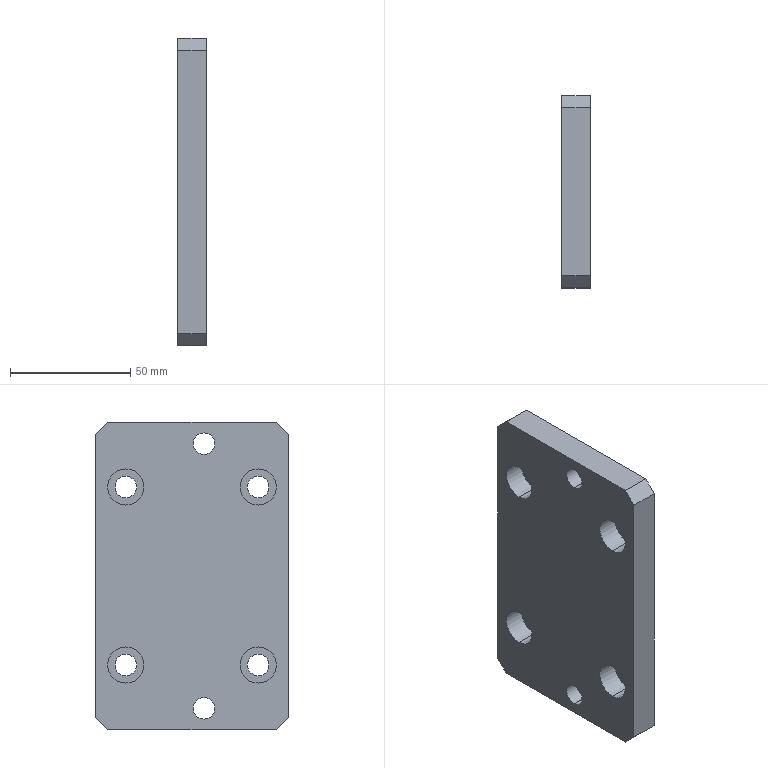Part | SolidWorks | features HoleWzd 2, Chamfer 1, Extrusion 1 | 1 solid | 34 faces | box 12 x 80 x 128 mm | volume 113628 mm3 | cylinder 20 | plane 14 | commonest cylinder face diameters 9 x12 15 x8
STEP:
#1=CARTESIAN_POINT('',(0.,-5.,59.5));
#2=VERTEX_POINT('',#1);
#3=CARTESIAN_POINT('',(0.,-5.,50.5));
#4=VERTEX_POINT('',#3);
#5=CARTESIAN_POINT('',(0.,-5.,55.));
#6=DIRECTION('',(1.,0.,0.));
#7=DIRECTION('',(0.,0.,-1.));
#8=AXIS2_PLACEMENT_3D('',#5,#6,#7);
#9=CIRCLE('',#8,4.5);
#10=EDGE_CURVE('',#2,#4,#9,.T.);
#11=ORIENTED_EDGE('',*,*,#10,.F.);
#12=CARTESIAN_POINT('',(12.,-5.,59.5));
#13=VERTEX_POINT('',#12);
#14=CARTESIAN_POINT('',(12.,-5.,59.5));
#15=DIRECTION('',(1.,0.,0.));
#16=VECTOR('',#15,1000.);
#17=LINE('',#14,#16);
#18=EDGE_CURVE('',#2,#13,#17,.T.);
#19=ORIENTED_EDGE('',*,*,#18,.T.);
#20=CARTESIAN_POINT('',(12.,-5.,50.5));
#21=VERTEX_POINT('',#20);
#22=CARTESIAN_POINT('',(12.,-5.,55.));
#23=DIRECTION('',(1.,0.,0.));
#24=DIRECTION('',(0.,0.,-1.));
#25=AXIS2_PLACEMENT_3D('',#22,#23,#24);
#26=CIRCLE('',#25,4.5);
#27=EDGE_CURVE('',#13,#21,#26,.T.);
#28=ORIENTED_EDGE('',*,*,#27,.T.);
#29=CARTESIAN_POINT('',(12.,-5.,50.5));
#30=DIRECTION('',(1.,0.,0.));
#31=VECTOR('',#30,1000.);
#32=LINE('',#29,#31);
#33=EDGE_CURVE('',#4,#21,#32,.T.);
#34=ORIENTED_EDGE('',*,*,#33,.F.);
#35=EDGE_LOOP('',(#11,#19,#28,#34));
#36=FACE_OUTER_BOUND('',#35,.T.);
#37=CARTESIAN_POINT('',(12.,-5.,55.));
#38=DIRECTION('',(1.,0.,0.));
#39=DIRECTION('',(0.,0.,-1.));
#40=AXIS2_PLACEMENT_3D('',#37,#38,#39);
#41=CYLINDRICAL_SURFACE('',#40,4.5);
#42=ADVANCED_FACE('',(#36),#41,.F.);
#43=CARTESIAN_POINT('',(0.,-5.,-50.5));
#44=VERTEX_POINT('',#43);
#45=CARTESIAN_POINT('',(0.,-5.,-59.5));
#46=VERTEX_POINT('',#45);
#47=CARTESIAN_POINT('',(0.,-5.,-55.));
#48=DIRECTION('',(1.,0.,0.));
#49=DIRECTION('',(0.,0.,-1.));
#50=AXIS2_PLACEMENT_3D('',#47,#48,#49);
#51=CIRCLE('',#50,4.5);
#52=EDGE_CURVE('',#44,#46,#51,.T.);
#53=ORIENTED_EDGE('',*,*,#52,.F.);
#54=CARTESIAN_POINT('',(12.,-5.,-50.5));
#55=VERTEX_POINT('',#54);
#56=CARTESIAN_POINT('',(12.,-5.,-50.5));
#57=DIRECTION('',(1.,0.,0.));
#58=VECTOR('',#57,1000.);
#59=LINE('',#56,#58);
#60=EDGE_CURVE('',#44,#55,#59,.T.);
#61=ORIENTED_EDGE('',*,*,#60,.T.);
#62=CARTESIAN_POINT('',(12.,-5.,-59.5));
#63=VERTEX_POINT('',#62);
#64=CARTESIAN_POINT('',(12.,-5.,-55.));
#65=DIRECTION('',(1.,0.,0.));
#66=DIRECTION('',(0.,0.,-1.));
#67=AXIS2_PLACEMENT_3D('',#64,#65,#66);
#68=CIRCLE('',#67,4.5);
#69=EDGE_CURVE('',#55,#63,#68,.T.);
#70=ORIENTED_EDGE('',*,*,#69,.T.);
#71=CARTESIAN_POINT('',(12.,-5.,-59.5));
#72=DIRECTION('',(1.,0.,0.));
#73=VECTOR('',#72,1000.);
#74=LINE('',#71,#73);
#75=EDGE_CURVE('',#46,#63,#74,.T.);
#76=ORIENTED_EDGE('',*,*,#75,.F.);
#77=EDGE_LOOP('',(#53,#61,#70,#76));
#78=FACE_OUTER_BOUND('',#77,.T.);
#79=CARTESIAN_POINT('',(12.,-5.,-55.));
#80=DIRECTION('',(1.,0.,0.));
#81=DIRECTION('',(0.,0.,-1.));
#82=AXIS2_PLACEMENT_3D('',#79,#80,#81);
#83=CYLINDRICAL_SURFACE('',#82,4.5);
#84=ADVANCED_FACE('',(#78),#83,.F.);
#85=CARTESIAN_POINT('',(9.,27.5,-44.5));
#86=VERTEX_POINT('',#85);
#87=CARTESIAN_POINT('',(9.,27.5,-29.5));
#88=VERTEX_POINT('',#87);
#89=CARTESIAN_POINT('',(9.,27.5,-37.));
#90=DIRECTION('',(-1.,0.,0.));
#91=DIRECTION('',(0.,0.,1.));
#92=AXIS2_PLACEMENT_3D('',#89,#90,#91);
#93=CIRCLE('',#92,7.5);
#94=EDGE_CURVE('',#86,#88,#93,.T.);
#95=ORIENTED_EDGE('',*,*,#94,.F.);
#96=CARTESIAN_POINT('',(0.,27.5,-44.5));
#97=VERTEX_POINT('',#96);
#98=CARTESIAN_POINT('',(0.,27.5,-44.5));
#99=DIRECTION('',(-1.,0.,0.));
#100=VECTOR('',#99,1000.);
#101=LINE('',#98,#100);
#102=EDGE_CURVE('',#86,#97,#101,.T.);
#103=ORIENTED_EDGE('',*,*,#102,.T.);
#104=CARTESIAN_POINT('',(0.,27.5,-29.5));
#105=VERTEX_POINT('',#104);
#106=CARTESIAN_POINT('',(0.,27.5,-37.));
#107=DIRECTION('',(-1.,0.,0.));
#108=DIRECTION('',(0.,0.,1.));
#109=AXIS2_PLACEMENT_3D('',#106,#107,#108);
#110=CIRCLE('',#109,7.5);
#111=EDGE_CURVE('',#97,#105,#110,.T.);
#112=ORIENTED_EDGE('',*,*,#111,.T.);
#113=CARTESIAN_POINT('',(0.,27.5,-29.5));
#114=DIRECTION('',(-1.,0.,0.));
#115=VECTOR('',#114,1000.);
#116=LINE('',#113,#115);
#117=EDGE_CURVE('',#88,#105,#116,.T.);
#118=ORIENTED_EDGE('',*,*,#117,.F.);
#119=EDGE_LOOP('',(#95,#103,#112,#118));
#120=FACE_OUTER_BOUND('',#119,.T.);
#121=CARTESIAN_POINT('',(0.,27.5,-37.));
#122=DIRECTION('',(-1.,0.,0.));
#123=DIRECTION('',(0.,0.,1.));
#124=AXIS2_PLACEMENT_3D('',#121,#122,#123);
#125=CYLINDRICAL_SURFACE('',#124,7.5);
#126=ADVANCED_FACE('',(#120),#125,.F.);
#127=CARTESIAN_POINT('',(12.,27.5,-41.5));
#128=VERTEX_POINT('',#127);
#129=CARTESIAN_POINT('',(12.,27.5,-32.5));
#130=VERTEX_POINT('',#129);
#131=CARTESIAN_POINT('',(12.,27.5,-37.));
#132=DIRECTION('',(-1.,0.,0.));
#133=DIRECTION('',(0.,0.,1.));
#134=AXIS2_PLACEMENT_3D('',#131,#132,#133);
#135=CIRCLE('',#134,4.5);
#136=EDGE_CURVE('',#128,#130,#135,.T.);
#137=ORIENTED_EDGE('',*,*,#136,.F.);
#138=CARTESIAN_POINT('',(9.,27.5,-41.5));
#139=VERTEX_POINT('',#138);
#140=CARTESIAN_POINT('',(0.,27.5,-41.5));
#141=DIRECTION('',(-1.,0.,0.));
#142=VECTOR('',#141,1000.);
#143=LINE('',#140,#142);
#144=EDGE_CURVE('',#128,#139,#143,.T.);
#145=ORIENTED_EDGE('',*,*,#144,.T.);
#146=CARTESIAN_POINT('',(9.,27.5,-32.5));
#147=VERTEX_POINT('',#146);
#148=CARTESIAN_POINT('',(9.,27.5,-37.));
#149=DIRECTION('',(-1.,0.,0.));
#150=DIRECTION('',(0.,0.,1.));
#151=AXIS2_PLACEMENT_3D('',#148,#149,#150);
#152=CIRCLE('',#151,4.5);
#153=EDGE_CURVE('',#139,#147,#152,.T.);
#154=ORIENTED_EDGE('',*,*,#153,.T.);
#155=CARTESIAN_POINT('',(0.,27.5,-32.5));
#156=DIRECTION('',(-1.,0.,0.));
#157=VECTOR('',#156,1000.);
#158=LINE('',#155,#157);
#159=EDGE_CURVE('',#130,#147,#158,.T.);
#160=ORIENTED_EDGE('',*,*,#159,.F.);
#161=EDGE_LOOP('',(#137,#145,#154,#160));
#162=FACE_OUTER_BOUND('',#161,.T.);
#163=CARTESIAN_POINT('',(0.,27.5,-37.));
#164=DIRECTION('',(-1.,0.,0.));
#165=DIRECTION('',(0.,0.,1.));
#166=AXIS2_PLACEMENT_3D('',#163,#164,#165);
#167=CYLINDRICAL_SURFACE('',#166,4.5);
#168=ADVANCED_FACE('',(#162),#167,.F.);
#169=CARTESIAN_POINT('',(9.,-27.5,-44.5));
#170=VERTEX_POINT('',#169);
#171=CARTESIAN_POINT('',(9.,-27.5,-29.5));
#172=VERTEX_POINT('',#171);
#173=CARTESIAN_POINT('',(9.,-27.5,-37.));
#174=DIRECTION('',(-1.,0.,0.));
#175=DIRECTION('',(0.,0.,1.));
#176=AXIS2_PLACEMENT_3D('',#173,#174,#175);
#177=CIRCLE('',#176,7.5);
#178=EDGE_CURVE('',#170,#172,#177,.T.);
#179=ORIENTED_EDGE('',*,*,#178,.F.);
#180=CARTESIAN_POINT('',(0.,-27.5,-44.5));
#181=VERTEX_POINT('',#180);
#182=CARTESIAN_POINT('',(0.,-27.5,-44.5));
#183=DIRECTION('',(-1.,0.,0.));
#184=VECTOR('',#183,1000.);
#185=LINE('',#182,#184);
#186=EDGE_CURVE('',#170,#181,#185,.T.);
#187=ORIENTED_EDGE('',*,*,#186,.T.);
#188=CARTESIAN_POINT('',(0.,-27.5,-29.5));
#189=VERTEX_POINT('',#188);
#190=CARTESIAN_POINT('',(0.,-27.5,-37.));
#191=DIRECTION('',(-1.,0.,0.));
#192=DIRECTION('',(0.,0.,1.));
#193=AXIS2_PLACEMENT_3D('',#190,#191,#192);
#194=CIRCLE('',#193,7.5);
#195=EDGE_CURVE('',#181,#189,#194,.T.);
#196=ORIENTED_EDGE('',*,*,#195,.T.);
#197=CARTESIAN_POINT('',(0.,-27.5,-29.5));
#198=DIRECTION('',(-1.,0.,0.));
#199=VECTOR('',#198,1000.);
#200=LINE('',#197,#199);
#201=EDGE_CURVE('',#172,#189,#200,.T.);
#202=ORIENTED_EDGE('',*,*,#201,.F.);
#203=EDGE_LOOP('',(#179,#187,#196,#202));
#204=FACE_OUTER_BOUND('',#203,.T.);
#205=CARTESIAN_POINT('',(0.,-27.5,-37.));
#206=DIRECTION('',(-1.,0.,0.));
#207=DIRECTION('',(0.,0.,1.));
#208=AXIS2_PLACEMENT_3D('',#205,#206,#207);
#209=CYLINDRICAL_SURFACE('',#208,7.5);
#210=ADVANCED_FACE('',(#204),#209,.F.);
#211=CARTESIAN_POINT('',(12.,-27.5,-41.5));
#212=VERTEX_POINT('',#211);
#213=CARTESIAN_POINT('',(12.,-27.5,-32.5));
#214=VERTEX_POINT('',#213);
#215=CARTESIAN_POINT('',(12.,-27.5,-37.));
#216=DIRECTION('',(-1.,0.,0.));
#217=DIRECTION('',(0.,0.,1.));
#218=AXIS2_PLACEMENT_3D('',#215,#216,#217);
#219=CIRCLE('',#218,4.5);
#220=EDGE_CURVE('',#212,#214,#219,.T.);
#221=ORIENTED_EDGE('',*,*,#220,.F.);
#222=CARTESIAN_POINT('',(9.,-27.5,-41.5));
#223=VERTEX_POINT('',#222);
#224=CARTESIAN_POINT('',(0.,-27.5,-41.5));
#225=DIRECTION('',(-1.,0.,0.));
#226=VECTOR('',#225,1000.);
#227=LINE('',#224,#226);
#228=EDGE_CURVE('',#212,#223,#227,.T.);
#229=ORIENTED_EDGE('',*,*,#228,.T.);
#230=CARTESIAN_POINT('',(9.,-27.5,-32.5));
#231=VERTEX_POINT('',#230);
#232=CARTESIAN_POINT('',(9.,-27.5,-37.));
#233=DIRECTION('',(-1.,0.,0.));
#234=DIRECTION('',(0.,0.,1.));
#235=AXIS2_PLACEMENT_3D('',#232,#233,#234);
#236=CIRCLE('',#235,4.5);
#237=EDGE_CURVE('',#223,#231,#236,.T.);
#238=ORIENTED_EDGE('',*,*,#237,.T.);
#239=CARTESIAN_POINT('',(0.,-27.5,-32.5));
#240=DIRECTION('',(-1.,0.,0.));
#241=VECTOR('',#240,1000.);
#242=LINE('',#239,#241);
#243=EDGE_CURVE('',#214,#231,#242,.T.);
#244=ORIENTED_EDGE('',*,*,#243,.F.);
#245=EDGE_LOOP('',(#221,#229,#238,#244));
#246=FACE_OUTER_BOUND('',#245,.T.);
#247=CARTESIAN_POINT('',(0.,-27.5,-37.));
#248=DIRECTION('',(-1.,0.,0.));
#249=DIRECTION('',(0.,0.,1.));
#250=AXIS2_PLACEMENT_3D('',#247,#248,#249);
#251=CYLINDRICAL_SURFACE('',#250,4.5);
#252=ADVANCED_FACE('',(#246),#251,.F.);
#253=CARTESIAN_POINT('',(9.,27.5,29.5));
#254=VERTEX_POINT('',#253);
#255=CARTESIAN_POINT('',(9.,27.5,44.5));
#256=VERTEX_POINT('',#255);
#257=CARTESIAN_POINT('',(9.,27.5,37.));
#258=DIRECTION('',(-1.,0.,0.));
#259=DIRECTION('',(0.,0.,1.));
#260=AXIS2_PLACEMENT_3D('',#257,#258,#259);
#261=CIRCLE('',#260,7.5);
#262=EDGE_CURVE('',#254,#256,#261,.T.);
#263=ORIENTED_EDGE('',*,*,#262,.F.);
#264=CARTESIAN_POINT('',(0.,27.5,29.5));
#265=VERTEX_POINT('',#264);
#266=CARTESIAN_POINT('',(0.,27.5,29.5));
#267=DIRECTION('',(-1.,0.,0.));
#268=VECTOR('',#267,1000.);
#269=LINE('',#266,#268);
#270=EDGE_CURVE('',#254,#265,#269,.T.);
#271=ORIENTED_EDGE('',*,*,#270,.T.);
#272=CARTESIAN_POINT('',(0.,27.5,44.5));
#273=VERTEX_POINT('',#272);
#274=CARTESIAN_POINT('',(0.,27.5,37.));
#275=DIRECTION('',(-1.,0.,0.));
#276=DIRECTION('',(0.,0.,1.));
#277=AXIS2_PLACEMENT_3D('',#274,#275,#276);
#278=CIRCLE('',#277,7.5);
#279=EDGE_CURVE('',#265,#273,#278,.T.);
#280=ORIENTED_EDGE('',*,*,#279,.T.);
#281=CARTESIAN_POINT('',(0.,27.5,44.5));
#282=DIRECTION('',(-1.,0.,0.));
#283=VECTOR('',#282,1000.);
#284=LINE('',#281,#283);
#285=EDGE_CURVE('',#256,#273,#284,.T.);
#286=ORIENTED_EDGE('',*,*,#285,.F.);
#287=EDGE_LOOP('',(#263,#271,#280,#286));
#288=FACE_OUTER_BOUND('',#287,.T.);
#289=CARTESIAN_POINT('',(0.,27.5,37.));
#290=DIRECTION('',(-1.,0.,0.));
#291=DIRECTION('',(0.,0.,1.));
#292=AXIS2_PLACEMENT_3D('',#289,#290,#291);
#293=CYLINDRICAL_SURFACE('',#292,7.5);
#294=ADVANCED_FACE('',(#288),#293,.F.);
#295=CARTESIAN_POINT('',(12.,27.5,32.5));
#296=VERTEX_POINT('',#295);
#297=CARTESIAN_POINT('',(12.,27.5,41.5));
#298=VERTEX_POINT('',#297);
#299=CARTESIAN_POINT('',(12.,27.5,37.));
#300=DIRECTION('',(-1.,0.,0.));
#301=DIRECTION('',(0.,0.,1.));
#302=AXIS2_PLACEMENT_3D('',#299,#300,#301);
#303=CIRCLE('',#302,4.5);
#304=EDGE_CURVE('',#296,#298,#303,.T.);
#305=ORIENTED_EDGE('',*,*,#304,.F.);
#306=CARTESIAN_POINT('',(9.,27.5,32.5));
#307=VERTEX_POINT('',#306);
#308=CARTESIAN_POINT('',(0.,27.5,32.5));
#309=DIRECTION('',(-1.,0.,0.));
#310=VECTOR('',#309,1000.);
#311=LINE('',#308,#310);
#312=EDGE_CURVE('',#296,#307,#311,.T.);
#313=ORIENTED_EDGE('',*,*,#312,.T.);
#314=CARTESIAN_POINT('',(9.,27.5,41.5));
#315=VERTEX_POINT('',#314);
#316=CARTESIAN_POINT('',(9.,27.5,37.));
#317=DIRECTION('',(-1.,0.,0.));
#318=DIRECTION('',(0.,0.,1.));
#319=AXIS2_PLACEMENT_3D('',#316,#317,#318);
#320=CIRCLE('',#319,4.5);
#321=EDGE_CURVE('',#307,#315,#320,.T.);
#322=ORIENTED_EDGE('',*,*,#321,.T.);
#323=CARTESIAN_POINT('',(0.,27.5,41.5));
#324=DIRECTION('',(-1.,0.,0.));
#325=VECTOR('',#324,1000.);
#326=LINE('',#323,#325);
#327=EDGE_CURVE('',#298,#315,#326,.T.);
#328=ORIENTED_EDGE('',*,*,#327,.F.);
#329=EDGE_LOOP('',(#305,#313,#322,#328));
#330=FACE_OUTER_BOUND('',#329,.T.);
#331=CARTESIAN_POINT('',(0.,27.5,37.));
#332=DIRECTION('',(-1.,0.,0.));
#333=DIRECTION('',(0.,0.,1.));
#334=AXIS2_PLACEMENT_3D('',#331,#332,#333);
#335=CYLINDRICAL_SURFACE('',#334,4.5);
#336=ADVANCED_FACE('',(#330),#335,.F.);
#337=CARTESIAN_POINT('',(9.,-27.5,29.5));
#338=VERTEX_POINT('',#337);
#339=CARTESIAN_POINT('',(9.,-27.5,44.5));
#340=VERTEX_POINT('',#339);
#341=CARTESIAN_POINT('',(9.,-27.5,37.));
#342=DIRECTION('',(-1.,0.,0.));
#343=DIRECTION('',(0.,0.,1.));
#344=AXIS2_PLACEMENT_3D('',#341,#342,#343);
#345=CIRCLE('',#344,7.5);
#346=EDGE_CURVE('',#338,#340,#345,.T.);
#347=ORIENTED_EDGE('',*,*,#346,.F.);
#348=CARTESIAN_POINT('',(0.,-27.5,29.5));
#349=VERTEX_POINT('',#348);
#350=CARTESIAN_POINT('',(0.,-27.5,29.5));
#351=DIRECTION('',(-1.,0.,0.));
#352=VECTOR('',#351,1000.);
#353=LINE('',#350,#352);
#354=EDGE_CURVE('',#338,#349,#353,.T.);
#355=ORIENTED_EDGE('',*,*,#354,.T.);
#356=CARTESIAN_POINT('',(0.,-27.5,44.5));
#357=VERTEX_POINT('',#356);
#358=CARTESIAN_POINT('',(0.,-27.5,37.));
#359=DIRECTION('',(-1.,0.,0.));
#360=DIRECTION('',(0.,0.,1.));
#361=AXIS2_PLACEMENT_3D('',#358,#359,#360);
#362=CIRCLE('',#361,7.5);
#363=EDGE_CURVE('',#349,#357,#362,.T.);
#364=ORIENTED_EDGE('',*,*,#363,.T.);
#365=CARTESIAN_POINT('',(0.,-27.5,44.5));
#366=DIRECTION('',(-1.,0.,0.));
#367=VECTOR('',#366,1000.);
#368=LINE('',#365,#367);
#369=EDGE_CURVE('',#340,#357,#368,.T.);
#370=ORIENTED_EDGE('',*,*,#369,.F.);
#371=EDGE_LOOP('',(#347,#355,#364,#370));
#372=FACE_OUTER_BOUND('',#371,.T.);
#373=CARTESIAN_POINT('',(0.,-27.5,37.));
#374=DIRECTION('',(-1.,0.,0.));
#375=DIRECTION('',(0.,0.,1.));
#376=AXIS2_PLACEMENT_3D('',#373,#374,#375);
#377=CYLINDRICAL_SURFACE('',#376,7.5);
#378=ADVANCED_FACE('',(#372),#377,.F.);
#379=CARTESIAN_POINT('',(12.,-27.5,32.5));
#380=VERTEX_POINT('',#379);
#381=CARTESIAN_POINT('',(12.,-27.5,41.5));
#382=VERTEX_POINT('',#381);
#383=CARTESIAN_POINT('',(12.,-27.5,37.));
#384=DIRECTION('',(-1.,0.,0.));
#385=DIRECTION('',(0.,0.,1.));
#386=AXIS2_PLACEMENT_3D('',#383,#384,#385);
#387=CIRCLE('',#386,4.5);
#388=EDGE_CURVE('',#380,#382,#387,.T.);
#389=ORIENTED_EDGE('',*,*,#388,.F.);
#390=CARTESIAN_POINT('',(9.,-27.5,32.5));
#391=VERTEX_POINT('',#390);
#392=CARTESIAN_POINT('',(0.,-27.5,32.5));
#393=DIRECTION('',(-1.,0.,0.));
#394=VECTOR('',#393,1000.);
#395=LINE('',#392,#394);
#396=EDGE_CURVE('',#380,#391,#395,.T.);
#397=ORIENTED_EDGE('',*,*,#396,.T.);
#398=CARTESIAN_POINT('',(9.,-27.5,41.5));
#399=VERTEX_POINT('',#398);
#400=CARTESIAN_POINT('',(9.,-27.5,37.));
#401=DIRECTION('',(-1.,0.,0.));
#402=DIRECTION('',(0.,0.,1.));
#403=AXIS2_PLACEMENT_3D('',#400,#401,#402);
#404=CIRCLE('',#403,4.5);
#405=EDGE_CURVE('',#391,#399,#404,.T.);
#406=ORIENTED_EDGE('',*,*,#405,.T.);
#407=CARTESIAN_POINT('',(0.,-27.5,41.5));
#408=DIRECTION('',(-1.,0.,0.));
#409=VECTOR('',#408,1000.);
#410=LINE('',#407,#409);
#411=EDGE_CURVE('',#382,#399,#410,.T.);
#412=ORIENTED_EDGE('',*,*,#411,.F.);
#413=EDGE_LOOP('',(#389,#397,#406,#412));
#414=FACE_OUTER_BOUND('',#413,.T.);
#415=CARTESIAN_POINT('',(0.,-27.5,37.));
#416=DIRECTION('',(-1.,0.,0.));
#417=DIRECTION('',(0.,0.,1.));
#418=AXIS2_PLACEMENT_3D('',#415,#416,#417);
#419=CYLINDRICAL_SURFACE('',#418,4.5);
#420=ADVANCED_FACE('',(#414),#419,.F.);
#421=CARTESIAN_POINT('',(12.,-35.,-64.));
#422=VERTEX_POINT('',#421);
#423=CARTESIAN_POINT('',(12.,35.,-64.));
#424=VERTEX_POINT('',#423);
#425=CARTESIAN_POINT('',(12.,40.,-64.));
#426=DIRECTION('',(0.,1.,0.));
#427=VECTOR('',#426,1000.);
#428=LINE('',#425,#427);
#429=EDGE_CURVE('',#422,#424,#428,.T.);
#430=ORIENTED_EDGE('',*,*,#429,.F.);
#431=CARTESIAN_POINT('',(0.,-35.,-64.));
#432=VERTEX_POINT('',#431);
#433=CARTESIAN_POINT('',(12.,-35.,-64.));
#434=DIRECTION('',(-1.,0.,0.));
#435=VECTOR('',#434,1000.);
#436=LINE('',#433,#435);
#437=EDGE_CURVE('',#422,#432,#436,.T.);
#438=ORIENTED_EDGE('',*,*,#437,.T.);
#439=CARTESIAN_POINT('',(0.,35.,-64.));
#440=VERTEX_POINT('',#439);
#441=CARTESIAN_POINT('',(0.,40.,-64.));
#442=DIRECTION('',(0.,1.,0.));
#443=VECTOR('',#442,1000.);
#444=LINE('',#441,#443);
#445=EDGE_CURVE('',#432,#440,#444,.T.);
#446=ORIENTED_EDGE('',*,*,#445,.T.);
#447=CARTESIAN_POINT('',(12.,35.,-64.));
#448=DIRECTION('',(1.,0.,0.));
#449=VECTOR('',#448,1000.);
#450=LINE('',#447,#449);
#451=EDGE_CURVE('',#440,#424,#450,.T.);
#452=ORIENTED_EDGE('',*,*,#451,.T.);
#453=EDGE_LOOP('',(#430,#438,#446,#452));
#454=FACE_OUTER_BOUND('',#453,.T.);
#455=CARTESIAN_POINT('',(12.,40.,-64.));
#456=DIRECTION('',(0.,0.,1.));
#457=DIRECTION('',(1.,0.,0.));
#458=AXIS2_PLACEMENT_3D('',#455,#456,#457);
#459=PLANE('',#458);
#460=ADVANCED_FACE('',(#454),#459,.F.);
#461=CARTESIAN_POINT('',(12.,40.,-59.));
#462=VERTEX_POINT('',#461);
#463=CARTESIAN_POINT('',(12.,40.,59.));
#464=VERTEX_POINT('',#463);
#465=CARTESIAN_POINT('',(12.,40.,64.));
#466=DIRECTION('',(0.,0.,1.));
#467=VECTOR('',#466,1000.);
#468=LINE('',#465,#467);
#469=EDGE_CURVE('',#462,#464,#468,.T.);
#470=ORIENTED_EDGE('',*,*,#469,.F.);
#471=CARTESIAN_POINT('',(0.,40.,-59.));
#472=VERTEX_POINT('',#471);
#473=CARTESIAN_POINT('',(12.,40.,-59.));
#474=DIRECTION('',(-1.,0.,0.));
#475=VECTOR('',#474,1000.);
#476=LINE('',#473,#475);
#477=EDGE_CURVE('',#462,#472,#476,.T.);
#478=ORIENTED_EDGE('',*,*,#477,.T.);
#479=CARTESIAN_POINT('',(0.,40.,59.));
#480=VERTEX_POINT('',#479);
#481=CARTESIAN_POINT('',(0.,40.,64.));
#482=DIRECTION('',(0.,0.,1.));
#483=VECTOR('',#482,1000.);
#484=LINE('',#481,#483);
#485=EDGE_CURVE('',#472,#480,#484,.T.);
#486=ORIENTED_EDGE('',*,*,#485,.T.);
#487=CARTESIAN_POINT('',(12.,40.,59.));
#488=DIRECTION('',(1.,0.,0.));
#489=VECTOR('',#488,1000.);
#490=LINE('',#487,#489);
#491=EDGE_CURVE('',#480,#464,#490,.T.);
#492=ORIENTED_EDGE('',*,*,#491,.T.);
#493=EDGE_LOOP('',(#470,#478,#486,#492));
#494=FACE_OUTER_BOUND('',#493,.T.);
#495=CARTESIAN_POINT('',(12.,40.,64.));
#496=DIRECTION('',(0.,-1.,0.));
#497=DIRECTION('',(0.,0.,-1.));
#498=AXIS2_PLACEMENT_3D('',#495,#496,#497);
#499=PLANE('',#498);
#500=ADVANCED_FACE('',(#494),#499,.F.);
#501=CARTESIAN_POINT('',(0.,35.,64.));
#502=VERTEX_POINT('',#501);
#503=CARTESIAN_POINT('',(0.,-35.,64.));
#504=VERTEX_POINT('',#503);
#505=CARTESIAN_POINT('',(0.,40.,64.));
#506=DIRECTION('',(0.,-1.,0.));
#507=VECTOR('',#506,1000.);
#508=LINE('',#505,#507);
#509=EDGE_CURVE('',#502,#504,#508,.T.);
#510=ORIENTED_EDGE('',*,*,#509,.T.);
#511=CARTESIAN_POINT('',(12.,-35.,64.));
#512=VERTEX_POINT('',#511);
#513=CARTESIAN_POINT('',(12.,-35.,64.));
#514=DIRECTION('',(1.,0.,0.));
#515=VECTOR('',#514,1000.);
#516=LINE('',#513,#515);
#517=EDGE_CURVE('',#504,#512,#516,.T.);
#518=ORIENTED_EDGE('',*,*,#517,.T.);
#519=CARTESIAN_POINT('',(12.,35.,64.));
#520=VERTEX_POINT('',#519);
#521=CARTESIAN_POINT('',(12.,40.,64.));
#522=DIRECTION('',(0.,-1.,0.));
#523=VECTOR('',#522,1000.);
#524=LINE('',#521,#523);
#525=EDGE_CURVE('',#520,#512,#524,.T.);
#526=ORIENTED_EDGE('',*,*,#525,.F.);
#527=CARTESIAN_POINT('',(12.,35.,64.));
#528=DIRECTION('',(-1.,0.,0.));
#529=VECTOR('',#528,1000.);
#530=LINE('',#527,#529);
#531=EDGE_CURVE('',#520,#502,#530,.T.);
#532=ORIENTED_EDGE('',*,*,#531,.T.);
#533=EDGE_LOOP('',(#510,#518,#526,#532));
#534=FACE_OUTER_BOUND('',#533,.T.);
#535=CARTESIAN_POINT('',(12.,40.,64.));
#536=DIRECTION('',(0.,0.,-1.));
#537=DIRECTION('',(0.,1.,0.));
#538=AXIS2_PLACEMENT_3D('',#535,#536,#537);
#539=PLANE('',#538);
#540=ADVANCED_FACE('',(#534),#539,.F.);
#541=CARTESIAN_POINT('',(12.,-40.,59.));
#542=VERTEX_POINT('',#541);
#543=CARTESIAN_POINT('',(12.,-40.,-59.));
#544=VERTEX_POINT('',#543);
#545=CARTESIAN_POINT('',(12.,-40.,64.));
#546=DIRECTION('',(0.,0.,-1.));
#547=VECTOR('',#546,1000.);
#548=LINE('',#545,#547);
#549=EDGE_CURVE('',#542,#544,#548,.T.);
#550=ORIENTED_EDGE('',*,*,#549,.F.);
#551=CARTESIAN_POINT('',(0.,-40.,59.));
#552=VERTEX_POINT('',#551);
#553=CARTESIAN_POINT('',(12.,-40.,59.));
#554=DIRECTION('',(-1.,0.,0.));
#555=VECTOR('',#554,1000.);
#556=LINE('',#553,#555);
#557=EDGE_CURVE('',#542,#552,#556,.T.);
#558=ORIENTED_EDGE('',*,*,#557,.T.);
#559=CARTESIAN_POINT('',(0.,-40.,-59.));
#560=VERTEX_POINT('',#559);
#561=CARTESIAN_POINT('',(0.,-40.,64.));
#562=DIRECTION('',(0.,0.,-1.));
#563=VECTOR('',#562,1000.);
#564=LINE('',#561,#563);
#565=EDGE_CURVE('',#552,#560,#564,.T.);
#566=ORIENTED_EDGE('',*,*,#565,.T.);
#567=CARTESIAN_POINT('',(12.,-40.,-59.));
#568=DIRECTION('',(1.,0.,0.));
#569=VECTOR('',#568,1000.);
#570=LINE('',#567,#569);
#571=EDGE_CURVE('',#560,#544,#570,.T.);
#572=ORIENTED_EDGE('',*,*,#571,.T.);
#573=EDGE_LOOP('',(#550,#558,#566,#572));
#574=FACE_OUTER_BOUND('',#573,.T.);
#575=CARTESIAN_POINT('',(12.,-40.,64.));
#576=DIRECTION('',(0.,1.,0.));
#577=DIRECTION('',(0.,0.,1.));
#578=AXIS2_PLACEMENT_3D('',#575,#576,#577);
#579=PLANE('',#578);
#580=ADVANCED_FACE('',(#574),#579,.F.);
#581=CARTESIAN_POINT('',(12.,-5.,55.));
#582=DIRECTION('',(1.,0.,0.));
#583=DIRECTION('',(0.,0.,-1.));
#584=AXIS2_PLACEMENT_3D('',#581,#582,#583);
#585=CIRCLE('',#584,4.5);
#586=EDGE_CURVE('',#21,#13,#585,.T.);
#587=ORIENTED_EDGE('',*,*,#586,.F.);
#588=ORIENTED_EDGE('',*,*,#27,.F.);
#589=EDGE_LOOP('',(#587,#588));
#590=FACE_BOUND('',#589,.T.);
#591=CARTESIAN_POINT('',(12.,-5.,-55.));
#592=DIRECTION('',(1.,0.,0.));
#593=DIRECTION('',(0.,0.,-1.));
#594=AXIS2_PLACEMENT_3D('',#591,#592,#593);
#595=CIRCLE('',#594,4.5);
#596=EDGE_CURVE('',#63,#55,#595,.T.);
#597=ORIENTED_EDGE('',*,*,#596,.F.);
#598=ORIENTED_EDGE('',*,*,#69,.F.);
#599=EDGE_LOOP('',(#597,#598));
#600=FACE_BOUND('',#599,.T.);
#601=CARTESIAN_POINT('',(12.,27.5,-37.));
#602=DIRECTION('',(-1.,0.,0.));
#603=DIRECTION('',(0.,0.,1.));
#604=AXIS2_PLACEMENT_3D('',#601,#602,#603);
#605=CIRCLE('',#604,4.5);
#606=EDGE_CURVE('',#130,#128,#605,.T.);
#607=ORIENTED_EDGE('',*,*,#606,.T.);
#608=ORIENTED_EDGE('',*,*,#136,.T.);
#609=EDGE_LOOP('',(#607,#608));
#610=FACE_BOUND('',#609,.T.);
#611=CARTESIAN_POINT('',(12.,-27.5,-37.));
#612=DIRECTION('',(-1.,0.,0.));
#613=DIRECTION('',(0.,0.,1.));
#614=AXIS2_PLACEMENT_3D('',#611,#612,#613);
#615=CIRCLE('',#614,4.5);
#616=EDGE_CURVE('',#214,#212,#615,.T.);
#617=ORIENTED_EDGE('',*,*,#616,.T.);
#618=ORIENTED_EDGE('',*,*,#220,.T.);
#619=EDGE_LOOP('',(#617,#618));
#620=FACE_BOUND('',#619,.T.);
#621=CARTESIAN_POINT('',(12.,27.5,37.));
#622=DIRECTION('',(-1.,0.,0.));
#623=DIRECTION('',(0.,0.,1.));
#624=AXIS2_PLACEMENT_3D('',#621,#622,#623);
#625=CIRCLE('',#624,4.5);
#626=EDGE_CURVE('',#298,#296,#625,.T.);
#627=ORIENTED_EDGE('',*,*,#626,.T.);
#628=ORIENTED_EDGE('',*,*,#304,.T.);
#629=EDGE_LOOP('',(#627,#628));
#630=FACE_BOUND('',#629,.T.);
#631=CARTESIAN_POINT('',(12.,-27.5,37.));
#632=DIRECTION('',(-1.,0.,0.));
#633=DIRECTION('',(0.,0.,1.));
#634=AXIS2_PLACEMENT_3D('',#631,#632,#633);
#635=CIRCLE('',#634,4.5);
#636=EDGE_CURVE('',#382,#380,#635,.T.);
#637=ORIENTED_EDGE('',*,*,#636,.T.);
#638=ORIENTED_EDGE('',*,*,#388,.T.);
#639=EDGE_LOOP('',(#637,#638));
#640=FACE_BOUND('',#639,.T.);
#641=ORIENTED_EDGE('',*,*,#525,.T.);
#642=CARTESIAN_POINT('',(12.,-49.5,49.5));
#643=DIRECTION('',(0.,-0.7071,-0.7071));
#644=VECTOR('',#643,1000.);
#645=LINE('',#642,#644);
#646=EDGE_CURVE('',#512,#542,#645,.T.);
#647=ORIENTED_EDGE('',*,*,#646,.T.);
#648=ORIENTED_EDGE('',*,*,#549,.T.);
#649=CARTESIAN_POINT('',(12.,-49.5,-49.5));
#650=DIRECTION('',(0.,0.7071,-0.7071));
#651=VECTOR('',#650,1000.);
#652=LINE('',#649,#651);
#653=EDGE_CURVE('',#544,#422,#652,.T.);
#654=ORIENTED_EDGE('',*,*,#653,.T.);
#655=ORIENTED_EDGE('',*,*,#429,.T.);
#656=CARTESIAN_POINT('',(12.,49.5,-49.5));
#657=DIRECTION('',(0.,0.7071,0.7071));
#658=VECTOR('',#657,1000.);
#659=LINE('',#656,#658);
#660=EDGE_CURVE('',#424,#462,#659,.T.);
#661=ORIENTED_EDGE('',*,*,#660,.T.);
#662=ORIENTED_EDGE('',*,*,#469,.T.);
#663=CARTESIAN_POINT('',(12.,49.5,49.5));
#664=DIRECTION('',(0.,-0.7071,0.7071));
#665=VECTOR('',#664,1000.);
#666=LINE('',#663,#665);
#667=EDGE_CURVE('',#464,#520,#666,.T.);
#668=ORIENTED_EDGE('',*,*,#667,.T.);
#669=EDGE_LOOP('',(#641,#647,#648,#654,#655,#661,#662,#668));
#670=FACE_OUTER_BOUND('',#669,.T.);
#671=CARTESIAN_POINT('',(12.,0.,0.));
#672=DIRECTION('',(1.,0.,0.));
#673=DIRECTION('',(0.,0.,-1.));
#674=AXIS2_PLACEMENT_3D('',#671,#672,#673);
#675=PLANE('',#674);
#676=ADVANCED_FACE('',(#590,#600,#610,#620,#630,#640,#670),#675,.T.);
#677=CARTESIAN_POINT('',(0.,-5.,55.));
#678=DIRECTION('',(1.,0.,0.));
#679=DIRECTION('',(0.,0.,-1.));
#680=AXIS2_PLACEMENT_3D('',#677,#678,#679);
#681=CIRCLE('',#680,4.5);
#682=EDGE_CURVE('',#4,#2,#681,.T.);
#683=ORIENTED_EDGE('',*,*,#682,.T.);
#684=ORIENTED_EDGE('',*,*,#10,.T.);
#685=EDGE_LOOP('',(#683,#684));
#686=FACE_BOUND('',#685,.T.);
#687=CARTESIAN_POINT('',(0.,-5.,-55.));
#688=DIRECTION('',(1.,0.,0.));
#689=DIRECTION('',(0.,0.,-1.));
#690=AXIS2_PLACEMENT_3D('',#687,#688,#689);
#691=CIRCLE('',#690,4.5);
#692=EDGE_CURVE('',#46,#44,#691,.T.);
#693=ORIENTED_EDGE('',*,*,#692,.T.);
#694=ORIENTED_EDGE('',*,*,#52,.T.);
#695=EDGE_LOOP('',(#693,#694));
#696=FACE_BOUND('',#695,.T.);
#697=CARTESIAN_POINT('',(0.,27.5,-37.));
#698=DIRECTION('',(-1.,0.,0.));
#699=DIRECTION('',(0.,0.,1.));
#700=AXIS2_PLACEMENT_3D('',#697,#698,#699);
#701=CIRCLE('',#700,7.5);
#702=EDGE_CURVE('',#105,#97,#701,.T.);
#703=ORIENTED_EDGE('',*,*,#702,.F.);
#704=ORIENTED_EDGE('',*,*,#111,.F.);
#705=EDGE_LOOP('',(#703,#704));
#706=FACE_BOUND('',#705,.T.);
#707=CARTESIAN_POINT('',(0.,-27.5,-37.));
#708=DIRECTION('',(-1.,0.,0.));
#709=DIRECTION('',(0.,0.,1.));
#710=AXIS2_PLACEMENT_3D('',#707,#708,#709);
#711=CIRCLE('',#710,7.5);
#712=EDGE_CURVE('',#189,#181,#711,.T.);
#713=ORIENTED_EDGE('',*,*,#712,.F.);
#714=ORIENTED_EDGE('',*,*,#195,.F.);
#715=EDGE_LOOP('',(#713,#714));
#716=FACE_BOUND('',#715,.T.);
#717=CARTESIAN_POINT('',(0.,27.5,37.));
#718=DIRECTION('',(-1.,0.,0.));
#719=DIRECTION('',(0.,0.,1.));
#720=AXIS2_PLACEMENT_3D('',#717,#718,#719);
#721=CIRCLE('',#720,7.5);
#722=EDGE_CURVE('',#273,#265,#721,.T.);
#723=ORIENTED_EDGE('',*,*,#722,.F.);
#724=ORIENTED_EDGE('',*,*,#279,.F.);
#725=EDGE_LOOP('',(#723,#724));
#726=FACE_BOUND('',#725,.T.);
#727=CARTESIAN_POINT('',(0.,-27.5,37.));
#728=DIRECTION('',(-1.,0.,0.));
#729=DIRECTION('',(0.,0.,1.));
#730=AXIS2_PLACEMENT_3D('',#727,#728,#729);
#731=CIRCLE('',#730,7.5);
#732=EDGE_CURVE('',#357,#349,#731,.T.);
#733=ORIENTED_EDGE('',*,*,#732,.F.);
#734=ORIENTED_EDGE('',*,*,#363,.F.);
#735=EDGE_LOOP('',(#733,#734));
#736=FACE_BOUND('',#735,.T.);
#737=ORIENTED_EDGE('',*,*,#565,.F.);
#738=CARTESIAN_POINT('',(0.,-40.,59.));
#739=DIRECTION('',(0.,0.7071,0.7071));
#740=VECTOR('',#739,1000.);
#741=LINE('',#738,#740);
#742=EDGE_CURVE('',#552,#504,#741,.T.);
#743=ORIENTED_EDGE('',*,*,#742,.T.);
#744=ORIENTED_EDGE('',*,*,#509,.F.);
#745=CARTESIAN_POINT('',(0.,35.,64.));
#746=DIRECTION('',(0.,0.7071,-0.7071));
#747=VECTOR('',#746,1000.);
#748=LINE('',#745,#747);
#749=EDGE_CURVE('',#502,#480,#748,.T.);
#750=ORIENTED_EDGE('',*,*,#749,.T.);
#751=ORIENTED_EDGE('',*,*,#485,.F.);
#752=CARTESIAN_POINT('',(0.,40.,-59.));
#753=DIRECTION('',(0.,-0.7071,-0.7071));
#754=VECTOR('',#753,1000.);
#755=LINE('',#752,#754);
#756=EDGE_CURVE('',#472,#440,#755,.T.);
#757=ORIENTED_EDGE('',*,*,#756,.T.);
#758=ORIENTED_EDGE('',*,*,#445,.F.);
#759=CARTESIAN_POINT('',(0.,-35.,-64.));
#760=DIRECTION('',(0.,-0.7071,0.7071));
#761=VECTOR('',#760,1000.);
#762=LINE('',#759,#761);
#763=EDGE_CURVE('',#432,#560,#762,.T.);
#764=ORIENTED_EDGE('',*,*,#763,.T.);
#765=EDGE_LOOP('',(#737,#743,#744,#750,#751,#757,#758,#764));
#766=FACE_OUTER_BOUND('',#765,.T.);
#767=CARTESIAN_POINT('',(0.,0.,0.));
#768=DIRECTION('',(1.,0.,0.));
#769=DIRECTION('',(0.,0.,-1.));
#770=AXIS2_PLACEMENT_3D('',#767,#768,#769);
#771=PLANE('',#770);
#772=ADVANCED_FACE('',(#686,#696,#706,#716,#726,#736,#766),#771,.F.);
#773=ORIENTED_EDGE('',*,*,#396,.F.);
#774=ORIENTED_EDGE('',*,*,#636,.F.);
#775=ORIENTED_EDGE('',*,*,#411,.T.);
#776=CARTESIAN_POINT('',(9.,-27.5,37.));
#777=DIRECTION('',(-1.,0.,0.));
#778=DIRECTION('',(0.,0.,1.));
#779=AXIS2_PLACEMENT_3D('',#776,#777,#778);
#780=CIRCLE('',#779,4.5);
#781=EDGE_CURVE('',#399,#391,#780,.T.);
#782=ORIENTED_EDGE('',*,*,#781,.T.);
#783=EDGE_LOOP('',(#773,#774,#775,#782));
#784=FACE_OUTER_BOUND('',#783,.T.);
#785=CARTESIAN_POINT('',(0.,-27.5,37.));
#786=DIRECTION('',(-1.,0.,0.));
#787=DIRECTION('',(0.,0.,1.));
#788=AXIS2_PLACEMENT_3D('',#785,#786,#787);
#789=CYLINDRICAL_SURFACE('',#788,4.5);
#790=ADVANCED_FACE('',(#784),#789,.F.);
#791=ORIENTED_EDGE('',*,*,#781,.F.);
#792=ORIENTED_EDGE('',*,*,#405,.F.);
#793=EDGE_LOOP('',(#791,#792));
#794=FACE_BOUND('',#793,.T.);
#795=CARTESIAN_POINT('',(9.,-27.5,37.));
#796=DIRECTION('',(-1.,0.,0.));
#797=DIRECTION('',(0.,0.,1.));
#798=AXIS2_PLACEMENT_3D('',#795,#796,#797);
#799=CIRCLE('',#798,7.5);
#800=EDGE_CURVE('',#340,#338,#799,.T.);
#801=ORIENTED_EDGE('',*,*,#800,.T.);
#802=ORIENTED_EDGE('',*,*,#346,.T.);
#803=EDGE_LOOP('',(#801,#802));
#804=FACE_OUTER_BOUND('',#803,.T.);
#805=CARTESIAN_POINT('',(9.,-23.,37.));
#806=DIRECTION('',(1.,0.,0.));
#807=DIRECTION('',(0.,0.,-1.));
#808=AXIS2_PLACEMENT_3D('',#805,#806,#807);
#809=PLANE('',#808);
#810=ADVANCED_FACE('',(#794,#804),#809,.F.);
#811=ORIENTED_EDGE('',*,*,#354,.F.);
#812=ORIENTED_EDGE('',*,*,#800,.F.);
#813=ORIENTED_EDGE('',*,*,#369,.T.);
#814=ORIENTED_EDGE('',*,*,#732,.T.);
#815=EDGE_LOOP('',(#811,#812,#813,#814));
#816=FACE_OUTER_BOUND('',#815,.T.);
#817=CARTESIAN_POINT('',(0.,-27.5,37.));
#818=DIRECTION('',(-1.,0.,0.));
#819=DIRECTION('',(0.,0.,1.));
#820=AXIS2_PLACEMENT_3D('',#817,#818,#819);
#821=CYLINDRICAL_SURFACE('',#820,7.5);
#822=ADVANCED_FACE('',(#816),#821,.F.);
#823=ORIENTED_EDGE('',*,*,#312,.F.);
#824=ORIENTED_EDGE('',*,*,#626,.F.);
#825=ORIENTED_EDGE('',*,*,#327,.T.);
#826=CARTESIAN_POINT('',(9.,27.5,37.));
#827=DIRECTION('',(-1.,0.,0.));
#828=DIRECTION('',(0.,0.,1.));
#829=AXIS2_PLACEMENT_3D('',#826,#827,#828);
#830=CIRCLE('',#829,4.5);
#831=EDGE_CURVE('',#315,#307,#830,.T.);
#832=ORIENTED_EDGE('',*,*,#831,.T.);
#833=EDGE_LOOP('',(#823,#824,#825,#832));
#834=FACE_OUTER_BOUND('',#833,.T.);
#835=CARTESIAN_POINT('',(0.,27.5,37.));
#836=DIRECTION('',(-1.,0.,0.));
#837=DIRECTION('',(0.,0.,1.));
#838=AXIS2_PLACEMENT_3D('',#835,#836,#837);
#839=CYLINDRICAL_SURFACE('',#838,4.5);
#840=ADVANCED_FACE('',(#834),#839,.F.);
#841=ORIENTED_EDGE('',*,*,#831,.F.);
#842=ORIENTED_EDGE('',*,*,#321,.F.);
#843=EDGE_LOOP('',(#841,#842));
#844=FACE_BOUND('',#843,.T.);
#845=CARTESIAN_POINT('',(9.,27.5,37.));
#846=DIRECTION('',(-1.,0.,0.));
#847=DIRECTION('',(0.,0.,1.));
#848=AXIS2_PLACEMENT_3D('',#845,#846,#847);
#849=CIRCLE('',#848,7.5);
#850=EDGE_CURVE('',#256,#254,#849,.T.);
#851=ORIENTED_EDGE('',*,*,#850,.T.);
#852=ORIENTED_EDGE('',*,*,#262,.T.);
#853=EDGE_LOOP('',(#851,#852));
#854=FACE_OUTER_BOUND('',#853,.T.);
#855=CARTESIAN_POINT('',(9.,32.,37.));
#856=DIRECTION('',(1.,0.,0.));
#857=DIRECTION('',(0.,0.,-1.));
#858=AXIS2_PLACEMENT_3D('',#855,#856,#857);
#859=PLANE('',#858);
#860=ADVANCED_FACE('',(#844,#854),#859,.F.);
#861=ORIENTED_EDGE('',*,*,#270,.F.);
#862=ORIENTED_EDGE('',*,*,#850,.F.);
#863=ORIENTED_EDGE('',*,*,#285,.T.);
#864=ORIENTED_EDGE('',*,*,#722,.T.);
#865=EDGE_LOOP('',(#861,#862,#863,#864));
#866=FACE_OUTER_BOUND('',#865,.T.);
#867=CARTESIAN_POINT('',(0.,27.5,37.));
#868=DIRECTION('',(-1.,0.,0.));
#869=DIRECTION('',(0.,0.,1.));
#870=AXIS2_PLACEMENT_3D('',#867,#868,#869);
#871=CYLINDRICAL_SURFACE('',#870,7.5);
#872=ADVANCED_FACE('',(#866),#871,.F.);
#873=ORIENTED_EDGE('',*,*,#228,.F.);
#874=ORIENTED_EDGE('',*,*,#616,.F.);
#875=ORIENTED_EDGE('',*,*,#243,.T.);
#876=CARTESIAN_POINT('',(9.,-27.5,-37.));
#877=DIRECTION('',(-1.,0.,0.));
#878=DIRECTION('',(0.,0.,1.));
#879=AXIS2_PLACEMENT_3D('',#876,#877,#878);
#880=CIRCLE('',#879,4.5);
#881=EDGE_CURVE('',#231,#223,#880,.T.);
#882=ORIENTED_EDGE('',*,*,#881,.T.);
#883=EDGE_LOOP('',(#873,#874,#875,#882));
#884=FACE_OUTER_BOUND('',#883,.T.);
#885=CARTESIAN_POINT('',(0.,-27.5,-37.));
#886=DIRECTION('',(-1.,0.,0.));
#887=DIRECTION('',(0.,0.,1.));
#888=AXIS2_PLACEMENT_3D('',#885,#886,#887);
#889=CYLINDRICAL_SURFACE('',#888,4.5);
#890=ADVANCED_FACE('',(#884),#889,.F.);
#891=ORIENTED_EDGE('',*,*,#881,.F.);
#892=ORIENTED_EDGE('',*,*,#237,.F.);
#893=EDGE_LOOP('',(#891,#892));
#894=FACE_BOUND('',#893,.T.);
#895=CARTESIAN_POINT('',(9.,-27.5,-37.));
#896=DIRECTION('',(-1.,0.,0.));
#897=DIRECTION('',(0.,0.,1.));
#898=AXIS2_PLACEMENT_3D('',#895,#896,#897);
#899=CIRCLE('',#898,7.5);
#900=EDGE_CURVE('',#172,#170,#899,.T.);
#901=ORIENTED_EDGE('',*,*,#900,.T.);
#902=ORIENTED_EDGE('',*,*,#178,.T.);
#903=EDGE_LOOP('',(#901,#902));
#904=FACE_OUTER_BOUND('',#903,.T.);
#905=CARTESIAN_POINT('',(9.,-23.,-37.));
#906=DIRECTION('',(1.,0.,0.));
#907=DIRECTION('',(0.,0.,-1.));
#908=AXIS2_PLACEMENT_3D('',#905,#906,#907);
#909=PLANE('',#908);
#910=ADVANCED_FACE('',(#894,#904),#909,.F.);
#911=ORIENTED_EDGE('',*,*,#186,.F.);
#912=ORIENTED_EDGE('',*,*,#900,.F.);
#913=ORIENTED_EDGE('',*,*,#201,.T.);
#914=ORIENTED_EDGE('',*,*,#712,.T.);
#915=EDGE_LOOP('',(#911,#912,#913,#914));
#916=FACE_OUTER_BOUND('',#915,.T.);
#917=CARTESIAN_POINT('',(0.,-27.5,-37.));
#918=DIRECTION('',(-1.,0.,0.));
#919=DIRECTION('',(0.,0.,1.));
#920=AXIS2_PLACEMENT_3D('',#917,#918,#919);
#921=CYLINDRICAL_SURFACE('',#920,7.5);
#922=ADVANCED_FACE('',(#916),#921,.F.);
#923=ORIENTED_EDGE('',*,*,#144,.F.);
#924=ORIENTED_EDGE('',*,*,#606,.F.);
#925=ORIENTED_EDGE('',*,*,#159,.T.);
#926=CARTESIAN_POINT('',(9.,27.5,-37.));
#927=DIRECTION('',(-1.,0.,0.));
#928=DIRECTION('',(0.,0.,1.));
#929=AXIS2_PLACEMENT_3D('',#926,#927,#928);
#930=CIRCLE('',#929,4.5);
#931=EDGE_CURVE('',#147,#139,#930,.T.);
#932=ORIENTED_EDGE('',*,*,#931,.T.);
#933=EDGE_LOOP('',(#923,#924,#925,#932));
#934=FACE_OUTER_BOUND('',#933,.T.);
#935=CARTESIAN_POINT('',(0.,27.5,-37.));
#936=DIRECTION('',(-1.,0.,0.));
#937=DIRECTION('',(0.,0.,1.));
#938=AXIS2_PLACEMENT_3D('',#935,#936,#937);
#939=CYLINDRICAL_SURFACE('',#938,4.5);
#940=ADVANCED_FACE('',(#934),#939,.F.);
#941=ORIENTED_EDGE('',*,*,#931,.F.);
#942=ORIENTED_EDGE('',*,*,#153,.F.);
#943=EDGE_LOOP('',(#941,#942));
#944=FACE_BOUND('',#943,.T.);
#945=CARTESIAN_POINT('',(9.,27.5,-37.));
#946=DIRECTION('',(-1.,0.,0.));
#947=DIRECTION('',(0.,0.,1.));
#948=AXIS2_PLACEMENT_3D('',#945,#946,#947);
#949=CIRCLE('',#948,7.5);
#950=EDGE_CURVE('',#88,#86,#949,.T.);
#951=ORIENTED_EDGE('',*,*,#950,.T.);
#952=ORIENTED_EDGE('',*,*,#94,.T.);
#953=EDGE_LOOP('',(#951,#952));
#954=FACE_OUTER_BOUND('',#953,.T.);
#955=CARTESIAN_POINT('',(9.,32.,-37.));
#956=DIRECTION('',(1.,0.,0.));
#957=DIRECTION('',(0.,0.,-1.));
#958=AXIS2_PLACEMENT_3D('',#955,#956,#957);
#959=PLANE('',#958);
#960=ADVANCED_FACE('',(#944,#954),#959,.F.);
#961=ORIENTED_EDGE('',*,*,#102,.F.);
#962=ORIENTED_EDGE('',*,*,#950,.F.);
#963=ORIENTED_EDGE('',*,*,#117,.T.);
#964=ORIENTED_EDGE('',*,*,#702,.T.);
#965=EDGE_LOOP('',(#961,#962,#963,#964));
#966=FACE_OUTER_BOUND('',#965,.T.);
#967=CARTESIAN_POINT('',(0.,27.5,-37.));
#968=DIRECTION('',(-1.,0.,0.));
#969=DIRECTION('',(0.,0.,1.));
#970=AXIS2_PLACEMENT_3D('',#967,#968,#969);
#971=CYLINDRICAL_SURFACE('',#970,7.5);
#972=ADVANCED_FACE('',(#966),#971,.F.);
#973=ORIENTED_EDGE('',*,*,#60,.F.);
#974=ORIENTED_EDGE('',*,*,#692,.F.);
#975=ORIENTED_EDGE('',*,*,#75,.T.);
#976=ORIENTED_EDGE('',*,*,#596,.T.);
#977=EDGE_LOOP('',(#973,#974,#975,#976));
#978=FACE_OUTER_BOUND('',#977,.T.);
#979=CARTESIAN_POINT('',(12.,-5.,-55.));
#980=DIRECTION('',(1.,0.,0.));
#981=DIRECTION('',(0.,0.,-1.));
#982=AXIS2_PLACEMENT_3D('',#979,#980,#981);
#983=CYLINDRICAL_SURFACE('',#982,4.5);
#984=ADVANCED_FACE('',(#978),#983,.F.);
#985=ORIENTED_EDGE('',*,*,#18,.F.);
#986=ORIENTED_EDGE('',*,*,#682,.F.);
#987=ORIENTED_EDGE('',*,*,#33,.T.);
#988=ORIENTED_EDGE('',*,*,#586,.T.);
#989=EDGE_LOOP('',(#985,#986,#987,#988));
#990=FACE_OUTER_BOUND('',#989,.T.);
#991=CARTESIAN_POINT('',(12.,-5.,55.));
#992=DIRECTION('',(1.,0.,0.));
#993=DIRECTION('',(0.,0.,-1.));
#994=AXIS2_PLACEMENT_3D('',#991,#992,#993);
#995=CYLINDRICAL_SURFACE('',#994,4.5);
#996=ADVANCED_FACE('',(#990),#995,.F.);
#997=ORIENTED_EDGE('',*,*,#646,.F.);
#998=ORIENTED_EDGE('',*,*,#517,.F.);
#999=ORIENTED_EDGE('',*,*,#742,.F.);
#1000=ORIENTED_EDGE('',*,*,#557,.F.);
#1001=EDGE_LOOP('',(#997,#998,#999,#1000));
#1002=FACE_OUTER_BOUND('',#1001,.T.);
#1003=CARTESIAN_POINT('',(12.,-40.,59.));
#1004=DIRECTION('',(0.,0.7071,-0.7071));
#1005=DIRECTION('',(-1.,0.,0.));
#1006=AXIS2_PLACEMENT_3D('',#1003,#1004,#1005);
#1007=PLANE('',#1006);
#1008=ADVANCED_FACE('',(#1002),#1007,.F.);
#1009=ORIENTED_EDGE('',*,*,#653,.F.);
#1010=ORIENTED_EDGE('',*,*,#571,.F.);
#1011=ORIENTED_EDGE('',*,*,#763,.F.);
#1012=ORIENTED_EDGE('',*,*,#437,.F.);
#1013=EDGE_LOOP('',(#1009,#1010,#1011,#1012));
#1014=FACE_OUTER_BOUND('',#1013,.T.);
#1015=CARTESIAN_POINT('',(12.,-35.,-64.));
#1016=DIRECTION('',(0.,0.7071,0.7071));
#1017=DIRECTION('',(-1.,0.,0.));
#1018=AXIS2_PLACEMENT_3D('',#1015,#1016,#1017);
#1019=PLANE('',#1018);
#1020=ADVANCED_FACE('',(#1014),#1019,.F.);
#1021=ORIENTED_EDGE('',*,*,#660,.F.);
#1022=ORIENTED_EDGE('',*,*,#451,.F.);
#1023=ORIENTED_EDGE('',*,*,#756,.F.);
#1024=ORIENTED_EDGE('',*,*,#477,.F.);
#1025=EDGE_LOOP('',(#1021,#1022,#1023,#1024));
#1026=FACE_OUTER_BOUND('',#1025,.T.);
#1027=CARTESIAN_POINT('',(12.,40.,-59.));
#1028=DIRECTION('',(0.,-0.7071,0.7071));
#1029=DIRECTION('',(-1.,0.,0.));
#1030=AXIS2_PLACEMENT_3D('',#1027,#1028,#1029);
#1031=PLANE('',#1030);
#1032=ADVANCED_FACE('',(#1026),#1031,.F.);
#1033=ORIENTED_EDGE('',*,*,#667,.F.);
#1034=ORIENTED_EDGE('',*,*,#491,.F.);
#1035=ORIENTED_EDGE('',*,*,#749,.F.);
#1036=ORIENTED_EDGE('',*,*,#531,.F.);
#1037=EDGE_LOOP('',(#1033,#1034,#1035,#1036));
#1038=FACE_OUTER_BOUND('',#1037,.T.);
#1039=CARTESIAN_POINT('',(12.,35.,64.));
#1040=DIRECTION('',(0.,-0.7071,-0.7071));
#1041=DIRECTION('',(-1.,0.,0.));
#1042=AXIS2_PLACEMENT_3D('',#1039,#1040,#1041);
#1043=PLANE('',#1042);
#1044=ADVANCED_FACE('',(#1038),#1043,.F.);
#1045=CLOSED_SHELL('',(#42,#84,#126,#168,#210,#252,#294,#336,#378,#420,#460,#500,#540,#580,#676,#772,#790,#810,#822,#840,#860,#872,#890,#910,#922,#940,#960,#972,#984,#996,#1008,#1020,#1032,#1044));
#1046=MANIFOLD_SOLID_BREP('',#1045);
#1047=CARTESIAN_POINT('',(0.,0.,0.));
#1048=DIRECTION('',(0.,0.,1.));
#1049=DIRECTION('',(1.,0.,0.));
#1050=AXIS2_PLACEMENT_3D('',#1047,#1048,#1049);
#1051=(LENGTH_UNIT()NAMED_UNIT(*)SI_UNIT(.MILLI.,.METRE.));
#1052=UNCERTAINTY_MEASURE_WITH_UNIT(LENGTH_MEASURE(0.00001),#1051,'','');
#1053=(NAMED_UNIT(*)PLANE_ANGLE_UNIT()SI_UNIT($,.RADIAN.));
#1054=(NAMED_UNIT(*)SI_UNIT($,.STERADIAN.)SOLID_ANGLE_UNIT());
#1055=(GEOMETRIC_REPRESENTATION_CONTEXT(3)GLOBAL_UNCERTAINTY_ASSIGNED_CONTEXT((#1052))GLOBAL_UNIT_ASSIGNED_CONTEXT((#1051,#1053,#1054))REPRESENTATION_CONTEXT('',''));
#1056=ADVANCED_BREP_SHAPE_REPRESENTATION('',(#1046,#1050),#1055);